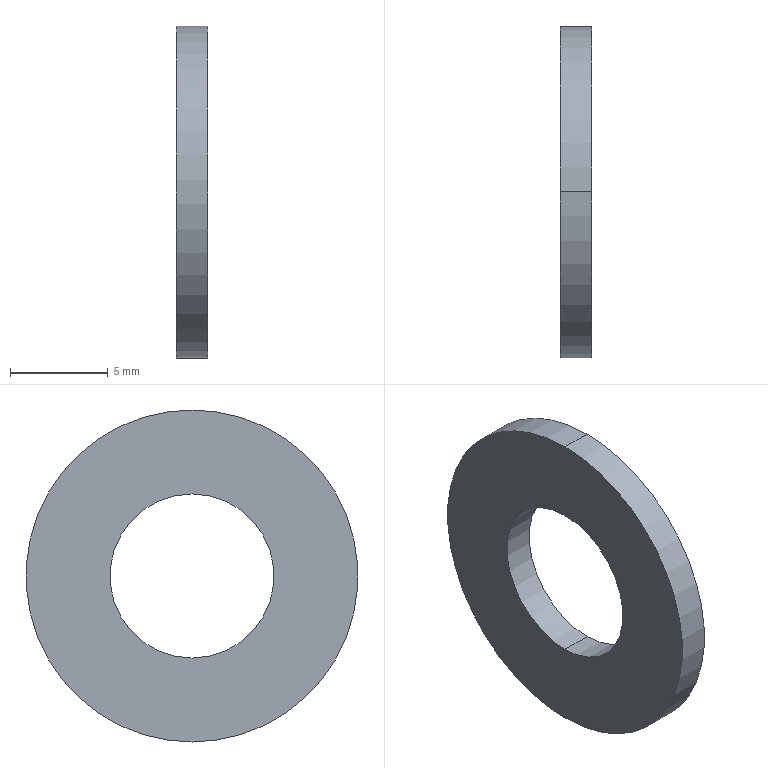Part | STEP file | 0228_314_SPWF8 | 1 solid | 6 faces | box 1.6 x 17 x 17 mm | volume 274.5 mm3 | cylinder 4 | plane 2 | commonest cylinder face diameters 8.4 x2 17 x2
STEP:
#1=CARTESIAN_POINT('',(0.,0.,0.));
#2=DIRECTION('',(0.,0.,1.));
#3=DIRECTION('',(1.,0.,0.));
#4=AXIS2_PLACEMENT_3D('',#1,#2,#3);
#5=CARTESIAN_POINT('',(-0.8,0.,-4.2));
#6=VERTEX_POINT('',#5);
#7=CARTESIAN_POINT('',(0.8,0.,-4.2));
#8=VERTEX_POINT('',#7);
#9=CARTESIAN_POINT('',(0.,0.,-4.2));
#10=DIRECTION('',(1.,0.,0.));
#11=VECTOR('',#10,1.);
#12=LINE('',#9,#11);
#13=CARTESIAN_POINT('',(0.,0.,0.));
#14=DIRECTION('',(1.,0.,0.));
#15=DIRECTION('',(0.,0.,-1.));
#16=AXIS2_PLACEMENT_3D('',#13,#14,#15);
#17=CYLINDRICAL_SURFACE('',#16,4.2);
#18=CARTESIAN_POINT('',(6.283,0.));
#19=DIRECTION('',(0.,1.));
#20=VECTOR('',#19,1.);
#21=LINE('',#18,#20);
#22=(GEOMETRIC_REPRESENTATION_CONTEXT(2)PARAMETRIC_REPRESENTATION_CONTEXT()REPRESENTATION_CONTEXT('',''));
#23=DEFINITIONAL_REPRESENTATION('',(#21),#22);
#24=PCURVE('',#17,#23);
#25=CARTESIAN_POINT('',(0.,0.,0.));
#26=DIRECTION('',(1.,0.,0.));
#27=DIRECTION('',(0.,0.,-1.));
#28=AXIS2_PLACEMENT_3D('',#25,#26,#27);
#29=CYLINDRICAL_SURFACE('',#28,4.2);
#30=CARTESIAN_POINT('',(0.,0.));
#31=DIRECTION('',(0.,1.));
#32=VECTOR('',#31,1.);
#33=LINE('',#30,#32);
#34=(GEOMETRIC_REPRESENTATION_CONTEXT(2)PARAMETRIC_REPRESENTATION_CONTEXT()REPRESENTATION_CONTEXT('',''));
#35=DEFINITIONAL_REPRESENTATION('',(#33),#34);
#36=PCURVE('',#29,#35);
#37=SURFACE_CURVE('',#12,(#24,#36),.PCURVE_S1.);
#38=EDGE_CURVE('',#6,#8,#37,.T.);
#39=ORIENTED_EDGE('',*,*,#38,.T.);
#40=CARTESIAN_POINT('',(0.8,0.,4.2));
#41=VERTEX_POINT('',#40);
#42=CARTESIAN_POINT('',(0.8,0.,0.));
#43=DIRECTION('',(-1.,0.,0.));
#44=DIRECTION('',(0.,0.,-1.));
#45=AXIS2_PLACEMENT_3D('',#42,#43,#44);
#46=CIRCLE('',#45,4.2);
#47=CARTESIAN_POINT('',(6.283,0.8));
#48=DIRECTION('',(-1.,0.));
#49=VECTOR('',#48,1.);
#50=LINE('',#47,#49);
#51=(GEOMETRIC_REPRESENTATION_CONTEXT(2)PARAMETRIC_REPRESENTATION_CONTEXT()REPRESENTATION_CONTEXT('',''));
#52=DEFINITIONAL_REPRESENTATION('',(#50),#51);
#53=PCURVE('',#17,#52);
#54=CARTESIAN_POINT('',(0.8,6.35,0.));
#55=DIRECTION('',(1.,0.,0.));
#56=DIRECTION('',(0.,0.,-1.));
#57=AXIS2_PLACEMENT_3D('',#54,#55,#56);
#58=PLANE('',#57);
#59=CARTESIAN_POINT('',(4.2,-6.35));
#60=CARTESIAN_POINT('',(4.2,-13.625));
#61=CARTESIAN_POINT('',(-2.1,-9.987));
#62=CARTESIAN_POINT('',(-8.4,-6.35));
#63=CARTESIAN_POINT('',(-2.1,-2.713));
#64=CARTESIAN_POINT('',(4.2,0.9246));
#65=CARTESIAN_POINT('',(4.2,-6.35));
#66=(BOUNDED_CURVE()B_SPLINE_CURVE(2,(#59,#60,#61,#62,#63,#64,#65),.UNSPECIFIED.,.T.,.F.)B_SPLINE_CURVE_WITH_KNOTS((1,2,2,2,2,1),(-2.094,0.,2.094,4.189,6.283,8.378),.UNSPECIFIED.)CURVE()GEOMETRIC_REPRESENTATION_ITEM()RATIONAL_B_SPLINE_CURVE((1.,0.5,1.,0.5,1.,0.5,1.))REPRESENTATION_ITEM(''));
#67=(GEOMETRIC_REPRESENTATION_CONTEXT(2)PARAMETRIC_REPRESENTATION_CONTEXT()REPRESENTATION_CONTEXT('',''));
#68=DEFINITIONAL_REPRESENTATION('',(#66),#67);
#69=PCURVE('',#58,#68);
#70=SURFACE_CURVE('',#46,(#53,#69),.PCURVE_S1.);
#71=EDGE_CURVE('',#8,#41,#70,.T.);
#72=ORIENTED_EDGE('',*,*,#71,.T.);
#73=CARTESIAN_POINT('',(-0.8,0.,4.2));
#74=VERTEX_POINT('',#73);
#75=CARTESIAN_POINT('',(0.,0.,4.2));
#76=DIRECTION('',(1.,0.,0.));
#77=VECTOR('',#76,1.);
#78=LINE('',#75,#77);
#79=CARTESIAN_POINT('',(3.142,0.));
#80=DIRECTION('',(0.,1.));
#81=VECTOR('',#80,1.);
#82=LINE('',#79,#81);
#83=(GEOMETRIC_REPRESENTATION_CONTEXT(2)PARAMETRIC_REPRESENTATION_CONTEXT()REPRESENTATION_CONTEXT('',''));
#84=DEFINITIONAL_REPRESENTATION('',(#82),#83);
#85=PCURVE('',#17,#84);
#86=CARTESIAN_POINT('',(3.142,0.));
#87=DIRECTION('',(0.,1.));
#88=VECTOR('',#87,1.);
#89=LINE('',#86,#88);
#90=(GEOMETRIC_REPRESENTATION_CONTEXT(2)PARAMETRIC_REPRESENTATION_CONTEXT()REPRESENTATION_CONTEXT('',''));
#91=DEFINITIONAL_REPRESENTATION('',(#89),#90);
#92=PCURVE('',#29,#91);
#93=SURFACE_CURVE('',#78,(#85,#92),.PCURVE_S1.);
#94=EDGE_CURVE('',#74,#41,#93,.T.);
#95=ORIENTED_EDGE('',*,*,#94,.F.);
#96=CARTESIAN_POINT('',(-0.8,0.,0.));
#97=DIRECTION('',(1.,0.,0.));
#98=DIRECTION('',(0.,0.,-1.));
#99=AXIS2_PLACEMENT_3D('',#96,#97,#98);
#100=CIRCLE('',#99,4.2);
#101=CARTESIAN_POINT('',(0.,-0.8));
#102=DIRECTION('',(1.,0.));
#103=VECTOR('',#102,1.);
#104=LINE('',#101,#103);
#105=(GEOMETRIC_REPRESENTATION_CONTEXT(2)PARAMETRIC_REPRESENTATION_CONTEXT()REPRESENTATION_CONTEXT('',''));
#106=DEFINITIONAL_REPRESENTATION('',(#104),#105);
#107=PCURVE('',#17,#106);
#108=CARTESIAN_POINT('',(-0.8,6.35,0.));
#109=DIRECTION('',(-1.,0.,0.));
#110=DIRECTION('',(0.,0.,1.));
#111=AXIS2_PLACEMENT_3D('',#108,#109,#110);
#112=PLANE('',#111);
#113=CARTESIAN_POINT('',(-4.2,-6.35));
#114=CARTESIAN_POINT('',(-4.2,0.9246));
#115=CARTESIAN_POINT('',(2.1,-2.713));
#116=CARTESIAN_POINT('',(8.4,-6.35));
#117=CARTESIAN_POINT('',(2.1,-9.987));
#118=CARTESIAN_POINT('',(-4.2,-13.625));
#119=CARTESIAN_POINT('',(-4.2,-6.35));
#120=(BOUNDED_CURVE()B_SPLINE_CURVE(2,(#113,#114,#115,#116,#117,#118,#119),.UNSPECIFIED.,.T.,.F.)B_SPLINE_CURVE_WITH_KNOTS((1,2,2,2,2,1),(-2.094,0.,2.094,4.189,6.283,8.378),.UNSPECIFIED.)CURVE()GEOMETRIC_REPRESENTATION_ITEM()RATIONAL_B_SPLINE_CURVE((1.,0.5,1.,0.5,1.,0.5,1.))REPRESENTATION_ITEM(''));
#121=(GEOMETRIC_REPRESENTATION_CONTEXT(2)PARAMETRIC_REPRESENTATION_CONTEXT()REPRESENTATION_CONTEXT('',''));
#122=DEFINITIONAL_REPRESENTATION('',(#120),#121);
#123=PCURVE('',#112,#122);
#124=SURFACE_CURVE('',#100,(#107,#123),.PCURVE_S1.);
#125=EDGE_CURVE('',#74,#6,#124,.T.);
#126=ORIENTED_EDGE('',*,*,#125,.T.);
#127=EDGE_LOOP('',(#39,#72,#95,#126));
#128=FACE_BOUND('',#127,.F.);
#129=ADVANCED_FACE('',(#128),#17,.F.);
#130=CARTESIAN_POINT('',(-0.8,0.,-8.5));
#131=VERTEX_POINT('',#130);
#132=CARTESIAN_POINT('',(-0.8,0.,8.5));
#133=VERTEX_POINT('',#132);
#134=CARTESIAN_POINT('',(-0.8,0.,0.));
#135=DIRECTION('',(1.,0.,0.));
#136=DIRECTION('',(0.,0.,-1.));
#137=AXIS2_PLACEMENT_3D('',#134,#135,#136);
#138=CIRCLE('',#137,8.5);
#139=CARTESIAN_POINT('',(0.,0.,0.));
#140=DIRECTION('',(1.,0.,0.));
#141=DIRECTION('',(0.,0.,-1.));
#142=AXIS2_PLACEMENT_3D('',#139,#140,#141);
#143=CYLINDRICAL_SURFACE('',#142,8.5);
#144=CARTESIAN_POINT('',(0.,-0.8));
#145=DIRECTION('',(1.,0.));
#146=VECTOR('',#145,1.);
#147=LINE('',#144,#146);
#148=(GEOMETRIC_REPRESENTATION_CONTEXT(2)PARAMETRIC_REPRESENTATION_CONTEXT()REPRESENTATION_CONTEXT('',''));
#149=DEFINITIONAL_REPRESENTATION('',(#147),#148);
#150=PCURVE('',#143,#149);
#151=CARTESIAN_POINT('',(-8.5,-6.35));
#152=CARTESIAN_POINT('',(-8.5,8.372));
#153=CARTESIAN_POINT('',(4.25,1.011));
#154=CARTESIAN_POINT('',(17.,-6.35));
#155=CARTESIAN_POINT('',(4.25,-13.711));
#156=CARTESIAN_POINT('',(-8.5,-21.072));
#157=CARTESIAN_POINT('',(-8.5,-6.35));
#158=(BOUNDED_CURVE()B_SPLINE_CURVE(2,(#151,#152,#153,#154,#155,#156,#157),.UNSPECIFIED.,.T.,.F.)B_SPLINE_CURVE_WITH_KNOTS((1,2,2,2,2,1),(-2.094,0.,2.094,4.189,6.283,8.378),.UNSPECIFIED.)CURVE()GEOMETRIC_REPRESENTATION_ITEM()RATIONAL_B_SPLINE_CURVE((1.,0.5,1.,0.5,1.,0.5,1.))REPRESENTATION_ITEM(''));
#159=(GEOMETRIC_REPRESENTATION_CONTEXT(2)PARAMETRIC_REPRESENTATION_CONTEXT()REPRESENTATION_CONTEXT('',''));
#160=DEFINITIONAL_REPRESENTATION('',(#158),#159);
#161=PCURVE('',#112,#160);
#162=SURFACE_CURVE('',#138,(#150,#161),.PCURVE_S1.);
#163=EDGE_CURVE('',#131,#133,#162,.T.);
#164=ORIENTED_EDGE('',*,*,#163,.T.);
#165=CARTESIAN_POINT('',(0.8,0.,8.5));
#166=VERTEX_POINT('',#165);
#167=CARTESIAN_POINT('',(0.,0.,8.5));
#168=DIRECTION('',(1.,0.,0.));
#169=VECTOR('',#168,1.);
#170=LINE('',#167,#169);
#171=CARTESIAN_POINT('',(3.142,0.));
#172=DIRECTION('',(0.,1.));
#173=VECTOR('',#172,1.);
#174=LINE('',#171,#173);
#175=(GEOMETRIC_REPRESENTATION_CONTEXT(2)PARAMETRIC_REPRESENTATION_CONTEXT()REPRESENTATION_CONTEXT('',''));
#176=DEFINITIONAL_REPRESENTATION('',(#174),#175);
#177=PCURVE('',#143,#176);
#178=CARTESIAN_POINT('',(0.,0.,0.));
#179=DIRECTION('',(1.,0.,0.));
#180=DIRECTION('',(0.,0.,-1.));
#181=AXIS2_PLACEMENT_3D('',#178,#179,#180);
#182=CYLINDRICAL_SURFACE('',#181,8.5);
#183=CARTESIAN_POINT('',(3.142,0.));
#184=DIRECTION('',(0.,1.));
#185=VECTOR('',#184,1.);
#186=LINE('',#183,#185);
#187=(GEOMETRIC_REPRESENTATION_CONTEXT(2)PARAMETRIC_REPRESENTATION_CONTEXT()REPRESENTATION_CONTEXT('',''));
#188=DEFINITIONAL_REPRESENTATION('',(#186),#187);
#189=PCURVE('',#182,#188);
#190=SURFACE_CURVE('',#170,(#177,#189),.PCURVE_S1.);
#191=EDGE_CURVE('',#133,#166,#190,.T.);
#192=ORIENTED_EDGE('',*,*,#191,.T.);
#193=CARTESIAN_POINT('',(0.8,0.,-8.5));
#194=VERTEX_POINT('',#193);
#195=CARTESIAN_POINT('',(0.8,0.,0.));
#196=DIRECTION('',(1.,0.,0.));
#197=DIRECTION('',(0.,0.,-1.));
#198=AXIS2_PLACEMENT_3D('',#195,#196,#197);
#199=CIRCLE('',#198,8.5);
#200=CARTESIAN_POINT('',(0.,0.8));
#201=DIRECTION('',(1.,0.));
#202=VECTOR('',#201,1.);
#203=LINE('',#200,#202);
#204=(GEOMETRIC_REPRESENTATION_CONTEXT(2)PARAMETRIC_REPRESENTATION_CONTEXT()REPRESENTATION_CONTEXT('',''));
#205=DEFINITIONAL_REPRESENTATION('',(#203),#204);
#206=PCURVE('',#143,#205);
#207=CARTESIAN_POINT('',(0.,-6.35));
#208=DIRECTION('',(1.,0.));
#209=AXIS2_PLACEMENT_2D('',#207,#208);
#210=CIRCLE('',#209,8.5);
#211=(GEOMETRIC_REPRESENTATION_CONTEXT(2)PARAMETRIC_REPRESENTATION_CONTEXT()REPRESENTATION_CONTEXT('',''));
#212=DEFINITIONAL_REPRESENTATION('',(#210),#211);
#213=PCURVE('',#58,#212);
#214=SURFACE_CURVE('',#199,(#206,#213),.PCURVE_S1.);
#215=EDGE_CURVE('',#194,#166,#214,.T.);
#216=ORIENTED_EDGE('',*,*,#215,.F.);
#217=CARTESIAN_POINT('',(0.,0.,-8.5));
#218=DIRECTION('',(1.,0.,0.));
#219=VECTOR('',#218,1.);
#220=LINE('',#217,#219);
#221=CARTESIAN_POINT('',(0.,0.));
#222=DIRECTION('',(0.,1.));
#223=VECTOR('',#222,1.);
#224=LINE('',#221,#223);
#225=(GEOMETRIC_REPRESENTATION_CONTEXT(2)PARAMETRIC_REPRESENTATION_CONTEXT()REPRESENTATION_CONTEXT('',''));
#226=DEFINITIONAL_REPRESENTATION('',(#224),#225);
#227=PCURVE('',#143,#226);
#228=CARTESIAN_POINT('',(6.283,0.));
#229=DIRECTION('',(0.,1.));
#230=VECTOR('',#229,1.);
#231=LINE('',#228,#230);
#232=(GEOMETRIC_REPRESENTATION_CONTEXT(2)PARAMETRIC_REPRESENTATION_CONTEXT()REPRESENTATION_CONTEXT('',''));
#233=DEFINITIONAL_REPRESENTATION('',(#231),#232);
#234=PCURVE('',#182,#233);
#235=SURFACE_CURVE('',#220,(#227,#234),.PCURVE_S1.);
#236=EDGE_CURVE('',#131,#194,#235,.T.);
#237=ORIENTED_EDGE('',*,*,#236,.F.);
#238=EDGE_LOOP('',(#164,#192,#216,#237));
#239=FACE_BOUND('',#238,.T.);
#240=ADVANCED_FACE('',(#239),#143,.T.);
#241=ORIENTED_EDGE('',*,*,#71,.T.);
#242=CARTESIAN_POINT('',(0.8,0.,0.));
#243=DIRECTION('',(-1.,0.,0.));
#244=DIRECTION('',(0.,0.,-1.));
#245=AXIS2_PLACEMENT_3D('',#242,#243,#244);
#246=CIRCLE('',#245,4.2);
#247=CARTESIAN_POINT('',(4.2,-6.35));
#248=CARTESIAN_POINT('',(4.2,-13.625));
#249=CARTESIAN_POINT('',(-2.1,-9.987));
#250=CARTESIAN_POINT('',(-8.4,-6.35));
#251=CARTESIAN_POINT('',(-2.1,-2.713));
#252=CARTESIAN_POINT('',(4.2,0.9246));
#253=CARTESIAN_POINT('',(4.2,-6.35));
#254=(BOUNDED_CURVE()B_SPLINE_CURVE(2,(#247,#248,#249,#250,#251,#252,#253),.UNSPECIFIED.,.T.,.F.)B_SPLINE_CURVE_WITH_KNOTS((1,2,2,2,2,1),(-2.094,0.,2.094,4.189,6.283,8.378),.UNSPECIFIED.)CURVE()GEOMETRIC_REPRESENTATION_ITEM()RATIONAL_B_SPLINE_CURVE((1.,0.5,1.,0.5,1.,0.5,1.))REPRESENTATION_ITEM(''));
#255=(GEOMETRIC_REPRESENTATION_CONTEXT(2)PARAMETRIC_REPRESENTATION_CONTEXT()REPRESENTATION_CONTEXT('',''));
#256=DEFINITIONAL_REPRESENTATION('',(#254),#255);
#257=PCURVE('',#58,#256);
#258=CARTESIAN_POINT('',(6.283,0.8));
#259=DIRECTION('',(-1.,0.));
#260=VECTOR('',#259,1.);
#261=LINE('',#258,#260);
#262=(GEOMETRIC_REPRESENTATION_CONTEXT(2)PARAMETRIC_REPRESENTATION_CONTEXT()REPRESENTATION_CONTEXT('',''));
#263=DEFINITIONAL_REPRESENTATION('',(#261),#262);
#264=PCURVE('',#29,#263);
#265=SURFACE_CURVE('',#246,(#257,#264),.PCURVE_S1.);
#266=EDGE_CURVE('',#41,#8,#265,.T.);
#267=ORIENTED_EDGE('',*,*,#266,.T.);
#268=EDGE_LOOP('',(#241,#267));
#269=FACE_BOUND('',#268,.T.);
#270=ORIENTED_EDGE('',*,*,#215,.T.);
#271=CARTESIAN_POINT('',(0.8,0.,0.));
#272=DIRECTION('',(1.,0.,0.));
#273=DIRECTION('',(0.,0.,-1.));
#274=AXIS2_PLACEMENT_3D('',#271,#272,#273);
#275=CIRCLE('',#274,8.5);
#276=CARTESIAN_POINT('',(0.,-6.35));
#277=DIRECTION('',(1.,0.));
#278=AXIS2_PLACEMENT_2D('',#276,#277);
#279=CIRCLE('',#278,8.5);
#280=(GEOMETRIC_REPRESENTATION_CONTEXT(2)PARAMETRIC_REPRESENTATION_CONTEXT()REPRESENTATION_CONTEXT('',''));
#281=DEFINITIONAL_REPRESENTATION('',(#279),#280);
#282=PCURVE('',#58,#281);
#283=CARTESIAN_POINT('',(0.,0.8));
#284=DIRECTION('',(1.,0.));
#285=VECTOR('',#284,1.);
#286=LINE('',#283,#285);
#287=(GEOMETRIC_REPRESENTATION_CONTEXT(2)PARAMETRIC_REPRESENTATION_CONTEXT()REPRESENTATION_CONTEXT('',''));
#288=DEFINITIONAL_REPRESENTATION('',(#286),#287);
#289=PCURVE('',#182,#288);
#290=SURFACE_CURVE('',#275,(#282,#289),.PCURVE_S1.);
#291=EDGE_CURVE('',#166,#194,#290,.T.);
#292=ORIENTED_EDGE('',*,*,#291,.T.);
#293=EDGE_LOOP('',(#270,#292));
#294=FACE_BOUND('',#293,.T.);
#295=ADVANCED_FACE('',(#269,#294),#58,.T.);
#296=ORIENTED_EDGE('',*,*,#266,.T.);
#297=ORIENTED_EDGE('',*,*,#38,.F.);
#298=CARTESIAN_POINT('',(-0.8,0.,0.));
#299=DIRECTION('',(1.,0.,0.));
#300=DIRECTION('',(0.,0.,-1.));
#301=AXIS2_PLACEMENT_3D('',#298,#299,#300);
#302=CIRCLE('',#301,4.2);
#303=CARTESIAN_POINT('',(0.,-0.8));
#304=DIRECTION('',(1.,0.));
#305=VECTOR('',#304,1.);
#306=LINE('',#303,#305);
#307=(GEOMETRIC_REPRESENTATION_CONTEXT(2)PARAMETRIC_REPRESENTATION_CONTEXT()REPRESENTATION_CONTEXT('',''));
#308=DEFINITIONAL_REPRESENTATION('',(#306),#307);
#309=PCURVE('',#29,#308);
#310=CARTESIAN_POINT('',(-4.2,-6.35));
#311=CARTESIAN_POINT('',(-4.2,0.9246));
#312=CARTESIAN_POINT('',(2.1,-2.713));
#313=CARTESIAN_POINT('',(8.4,-6.35));
#314=CARTESIAN_POINT('',(2.1,-9.987));
#315=CARTESIAN_POINT('',(-4.2,-13.625));
#316=CARTESIAN_POINT('',(-4.2,-6.35));
#317=(BOUNDED_CURVE()B_SPLINE_CURVE(2,(#310,#311,#312,#313,#314,#315,#316),.UNSPECIFIED.,.T.,.F.)B_SPLINE_CURVE_WITH_KNOTS((1,2,2,2,2,1),(-2.094,0.,2.094,4.189,6.283,8.378),.UNSPECIFIED.)CURVE()GEOMETRIC_REPRESENTATION_ITEM()RATIONAL_B_SPLINE_CURVE((1.,0.5,1.,0.5,1.,0.5,1.))REPRESENTATION_ITEM(''));
#318=(GEOMETRIC_REPRESENTATION_CONTEXT(2)PARAMETRIC_REPRESENTATION_CONTEXT()REPRESENTATION_CONTEXT('',''));
#319=DEFINITIONAL_REPRESENTATION('',(#317),#318);
#320=PCURVE('',#112,#319);
#321=SURFACE_CURVE('',#302,(#309,#320),.PCURVE_S1.);
#322=EDGE_CURVE('',#6,#74,#321,.T.);
#323=ORIENTED_EDGE('',*,*,#322,.T.);
#324=ORIENTED_EDGE('',*,*,#94,.T.);
#325=EDGE_LOOP('',(#296,#297,#323,#324));
#326=FACE_BOUND('',#325,.F.);
#327=ADVANCED_FACE('',(#326),#29,.F.);
#328=ORIENTED_EDGE('',*,*,#191,.F.);
#329=CARTESIAN_POINT('',(-0.8,0.,0.));
#330=DIRECTION('',(1.,0.,0.));
#331=DIRECTION('',(0.,0.,-1.));
#332=AXIS2_PLACEMENT_3D('',#329,#330,#331);
#333=CIRCLE('',#332,8.5);
#334=CARTESIAN_POINT('',(0.,-0.8));
#335=DIRECTION('',(1.,0.));
#336=VECTOR('',#335,1.);
#337=LINE('',#334,#336);
#338=(GEOMETRIC_REPRESENTATION_CONTEXT(2)PARAMETRIC_REPRESENTATION_CONTEXT()REPRESENTATION_CONTEXT('',''));
#339=DEFINITIONAL_REPRESENTATION('',(#337),#338);
#340=PCURVE('',#182,#339);
#341=CARTESIAN_POINT('',(-8.5,-6.35));
#342=CARTESIAN_POINT('',(-8.5,8.372));
#343=CARTESIAN_POINT('',(4.25,1.011));
#344=CARTESIAN_POINT('',(17.,-6.35));
#345=CARTESIAN_POINT('',(4.25,-13.711));
#346=CARTESIAN_POINT('',(-8.5,-21.072));
#347=CARTESIAN_POINT('',(-8.5,-6.35));
#348=(BOUNDED_CURVE()B_SPLINE_CURVE(2,(#341,#342,#343,#344,#345,#346,#347),.UNSPECIFIED.,.T.,.F.)B_SPLINE_CURVE_WITH_KNOTS((1,2,2,2,2,1),(-2.094,0.,2.094,4.189,6.283,8.378),.UNSPECIFIED.)CURVE()GEOMETRIC_REPRESENTATION_ITEM()RATIONAL_B_SPLINE_CURVE((1.,0.5,1.,0.5,1.,0.5,1.))REPRESENTATION_ITEM(''));
#349=(GEOMETRIC_REPRESENTATION_CONTEXT(2)PARAMETRIC_REPRESENTATION_CONTEXT()REPRESENTATION_CONTEXT('',''));
#350=DEFINITIONAL_REPRESENTATION('',(#348),#349);
#351=PCURVE('',#112,#350);
#352=SURFACE_CURVE('',#333,(#340,#351),.PCURVE_S1.);
#353=EDGE_CURVE('',#133,#131,#352,.T.);
#354=ORIENTED_EDGE('',*,*,#353,.T.);
#355=ORIENTED_EDGE('',*,*,#236,.T.);
#356=ORIENTED_EDGE('',*,*,#291,.F.);
#357=EDGE_LOOP('',(#328,#354,#355,#356));
#358=FACE_BOUND('',#357,.T.);
#359=ADVANCED_FACE('',(#358),#182,.T.);
#360=ORIENTED_EDGE('',*,*,#163,.F.);
#361=ORIENTED_EDGE('',*,*,#353,.F.);
#362=EDGE_LOOP('',(#360,#361));
#363=FACE_BOUND('',#362,.T.);
#364=ORIENTED_EDGE('',*,*,#322,.T.);
#365=ORIENTED_EDGE('',*,*,#125,.T.);
#366=EDGE_LOOP('',(#364,#365));
#367=FACE_BOUND('',#366,.T.);
#368=ADVANCED_FACE('',(#363,#367),#112,.T.);
#369=CLOSED_SHELL('',(#129,#240,#295,#327,#359,#368));
#370=MANIFOLD_SOLID_BREP('',#369);
#371=(LENGTH_UNIT()NAMED_UNIT(*)SI_UNIT(.MILLI.,.METRE.));
#372=UNCERTAINTY_MEASURE_WITH_UNIT(LENGTH_MEASURE(0.0000001),#371,'','');
#373=(NAMED_UNIT(*)PLANE_ANGLE_UNIT()SI_UNIT($,.RADIAN.));
#374=(NAMED_UNIT(*)SI_UNIT($,.STERADIAN.)SOLID_ANGLE_UNIT());
#375=(GEOMETRIC_REPRESENTATION_CONTEXT(3)GLOBAL_UNCERTAINTY_ASSIGNED_CONTEXT((#372))GLOBAL_UNIT_ASSIGNED_CONTEXT((#371,#373,#374))REPRESENTATION_CONTEXT('',''));
#376=ADVANCED_BREP_SHAPE_REPRESENTATION('',(#4,#370),#375);